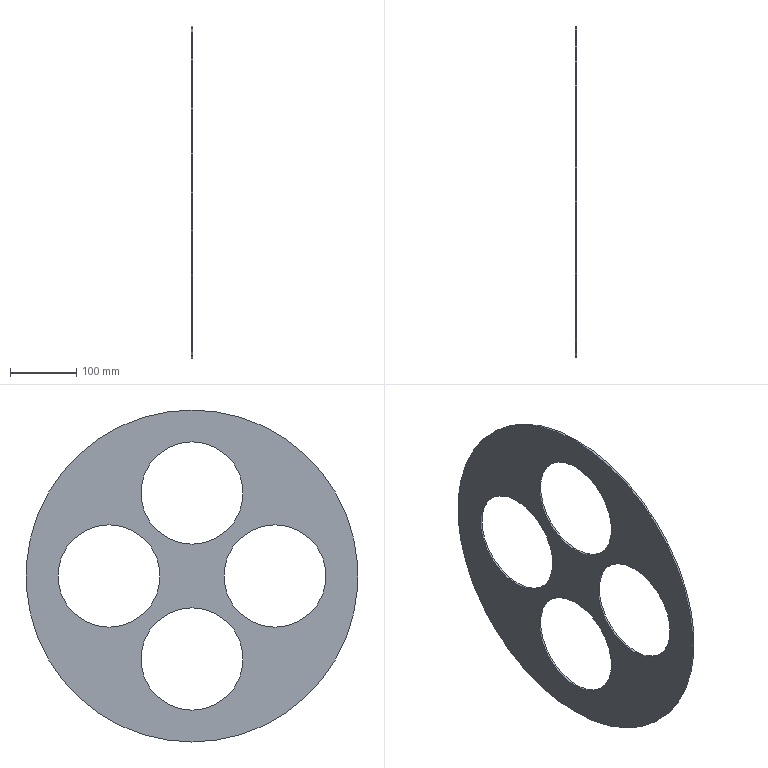Part | SolidWorks | features CirPattern 2, ICE 2, Extrusion 1 | 1 solid | 12 faces | box 3 x 500 x 500 mm | volume 365531 mm3 | cylinder 10 | plane 2 | commonest cylinder face diameters 154 x8 500 x2
STEP:
#1=CARTESIAN_POINT('',(0.,0.,-48.));
#2=VERTEX_POINT('',#1);
#3=CARTESIAN_POINT('',(0.,0.,-202.));
#4=VERTEX_POINT('',#3);
#5=CARTESIAN_POINT('',(0.,0.,-125.));
#6=DIRECTION('',(1.,0.,0.));
#7=DIRECTION('',(0.,0.,-1.));
#8=AXIS2_PLACEMENT_3D('',#5,#6,#7);
#9=CIRCLE('',#8,77.);
#10=EDGE_CURVE('',#2,#4,#9,.T.);
#11=ORIENTED_EDGE('',*,*,#10,.F.);
#12=CARTESIAN_POINT('',(3.,0.,-48.));
#13=VERTEX_POINT('',#12);
#14=CARTESIAN_POINT('',(-7.,0.,-48.));
#15=DIRECTION('',(1.,0.,0.));
#16=VECTOR('',#15,1000.);
#17=LINE('',#14,#16);
#18=EDGE_CURVE('',#2,#13,#17,.T.);
#19=ORIENTED_EDGE('',*,*,#18,.T.);
#20=CARTESIAN_POINT('',(3.,0.,-202.));
#21=VERTEX_POINT('',#20);
#22=CARTESIAN_POINT('',(3.,0.,-125.));
#23=DIRECTION('',(1.,0.,0.));
#24=DIRECTION('',(0.,-1.,0.));
#25=AXIS2_PLACEMENT_3D('',#22,#23,#24);
#26=CIRCLE('',#25,77.);
#27=EDGE_CURVE('',#13,#21,#26,.T.);
#28=ORIENTED_EDGE('',*,*,#27,.T.);
#29=CARTESIAN_POINT('',(-7.,0.,-202.));
#30=DIRECTION('',(1.,0.,0.));
#31=VECTOR('',#30,1000.);
#32=LINE('',#29,#31);
#33=EDGE_CURVE('',#4,#21,#32,.T.);
#34=ORIENTED_EDGE('',*,*,#33,.F.);
#35=EDGE_LOOP('',(#11,#19,#28,#34));
#36=FACE_OUTER_BOUND('',#35,.T.);
#37=CARTESIAN_POINT('',(-7.,0.,-125.));
#38=DIRECTION('',(1.,0.,0.));
#39=DIRECTION('',(0.,0.,-1.));
#40=AXIS2_PLACEMENT_3D('',#37,#38,#39);
#41=CYLINDRICAL_SURFACE('',#40,77.);
#42=ADVANCED_FACE('',(#36),#41,.F.);
#43=CARTESIAN_POINT('',(0.,-125.,77.));
#44=VERTEX_POINT('',#43);
#45=CARTESIAN_POINT('',(0.,-125.,-77.));
#46=VERTEX_POINT('',#45);
#47=CARTESIAN_POINT('',(0.,-125.,0.));
#48=DIRECTION('',(1.,0.,0.));
#49=DIRECTION('',(0.,0.,-1.));
#50=AXIS2_PLACEMENT_3D('',#47,#48,#49);
#51=CIRCLE('',#50,77.);
#52=EDGE_CURVE('',#44,#46,#51,.T.);
#53=ORIENTED_EDGE('',*,*,#52,.F.);
#54=CARTESIAN_POINT('',(3.,-125.,77.));
#55=VERTEX_POINT('',#54);
#56=CARTESIAN_POINT('',(-7.,-125.,77.));
#57=DIRECTION('',(1.,0.,0.));
#58=VECTOR('',#57,1000.);
#59=LINE('',#56,#58);
#60=EDGE_CURVE('',#44,#55,#59,.T.);
#61=ORIENTED_EDGE('',*,*,#60,.T.);
#62=CARTESIAN_POINT('',(3.,-125.,-77.));
#63=VERTEX_POINT('',#62);
#64=CARTESIAN_POINT('',(3.,-125.,0.));
#65=DIRECTION('',(1.,0.,0.));
#66=DIRECTION('',(0.,0.,1.));
#67=AXIS2_PLACEMENT_3D('',#64,#65,#66);
#68=CIRCLE('',#67,77.);
#69=EDGE_CURVE('',#55,#63,#68,.T.);
#70=ORIENTED_EDGE('',*,*,#69,.T.);
#71=CARTESIAN_POINT('',(-7.,-125.,-77.));
#72=DIRECTION('',(1.,0.,0.));
#73=VECTOR('',#72,1000.);
#74=LINE('',#71,#73);
#75=EDGE_CURVE('',#46,#63,#74,.T.);
#76=ORIENTED_EDGE('',*,*,#75,.F.);
#77=EDGE_LOOP('',(#53,#61,#70,#76));
#78=FACE_OUTER_BOUND('',#77,.T.);
#79=CARTESIAN_POINT('',(-7.,-125.,0.));
#80=DIRECTION('',(1.,0.,0.));
#81=DIRECTION('',(0.,0.,-1.));
#82=AXIS2_PLACEMENT_3D('',#79,#80,#81);
#83=CYLINDRICAL_SURFACE('',#82,77.);
#84=ADVANCED_FACE('',(#78),#83,.F.);
#85=CARTESIAN_POINT('',(0.,0.,202.));
#86=VERTEX_POINT('',#85);
#87=CARTESIAN_POINT('',(0.,0.,48.));
#88=VERTEX_POINT('',#87);
#89=CARTESIAN_POINT('',(0.,0.,125.));
#90=DIRECTION('',(1.,0.,0.));
#91=DIRECTION('',(0.,0.,-1.));
#92=AXIS2_PLACEMENT_3D('',#89,#90,#91);
#93=CIRCLE('',#92,77.);
#94=EDGE_CURVE('',#86,#88,#93,.T.);
#95=ORIENTED_EDGE('',*,*,#94,.F.);
#96=CARTESIAN_POINT('',(3.,0.,202.));
#97=VERTEX_POINT('',#96);
#98=CARTESIAN_POINT('',(-7.,0.,202.));
#99=DIRECTION('',(1.,0.,0.));
#100=VECTOR('',#99,1000.);
#101=LINE('',#98,#100);
#102=EDGE_CURVE('',#86,#97,#101,.T.);
#103=ORIENTED_EDGE('',*,*,#102,.T.);
#104=CARTESIAN_POINT('',(3.,0.,48.));
#105=VERTEX_POINT('',#104);
#106=CARTESIAN_POINT('',(3.,0.,125.));
#107=DIRECTION('',(1.,0.,0.));
#108=DIRECTION('',(0.,1.,0.));
#109=AXIS2_PLACEMENT_3D('',#106,#107,#108);
#110=CIRCLE('',#109,77.);
#111=EDGE_CURVE('',#97,#105,#110,.T.);
#112=ORIENTED_EDGE('',*,*,#111,.T.);
#113=CARTESIAN_POINT('',(-7.,0.,48.));
#114=DIRECTION('',(1.,0.,0.));
#115=VECTOR('',#114,1000.);
#116=LINE('',#113,#115);
#117=EDGE_CURVE('',#88,#105,#116,.T.);
#118=ORIENTED_EDGE('',*,*,#117,.F.);
#119=EDGE_LOOP('',(#95,#103,#112,#118));
#120=FACE_OUTER_BOUND('',#119,.T.);
#121=CARTESIAN_POINT('',(-7.,0.,125.));
#122=DIRECTION('',(1.,0.,0.));
#123=DIRECTION('',(0.,0.,-1.));
#124=AXIS2_PLACEMENT_3D('',#121,#122,#123);
#125=CYLINDRICAL_SURFACE('',#124,77.);
#126=ADVANCED_FACE('',(#120),#125,.F.);
#127=CARTESIAN_POINT('',(0.,125.,77.));
#128=VERTEX_POINT('',#127);
#129=CARTESIAN_POINT('',(0.,125.,-77.));
#130=VERTEX_POINT('',#129);
#131=CARTESIAN_POINT('',(0.,125.,0.));
#132=DIRECTION('',(1.,0.,0.));
#133=DIRECTION('',(0.,0.,-1.));
#134=AXIS2_PLACEMENT_3D('',#131,#132,#133);
#135=CIRCLE('',#134,77.);
#136=EDGE_CURVE('',#128,#130,#135,.T.);
#137=ORIENTED_EDGE('',*,*,#136,.F.);
#138=CARTESIAN_POINT('',(3.,125.,77.));
#139=VERTEX_POINT('',#138);
#140=CARTESIAN_POINT('',(-7.,125.,77.));
#141=DIRECTION('',(1.,0.,0.));
#142=VECTOR('',#141,1000.);
#143=LINE('',#140,#142);
#144=EDGE_CURVE('',#128,#139,#143,.T.);
#145=ORIENTED_EDGE('',*,*,#144,.T.);
#146=CARTESIAN_POINT('',(3.,125.,-77.));
#147=VERTEX_POINT('',#146);
#148=CARTESIAN_POINT('',(3.,125.,0.));
#149=DIRECTION('',(1.,0.,0.));
#150=DIRECTION('',(0.,0.,-1.));
#151=AXIS2_PLACEMENT_3D('',#148,#149,#150);
#152=CIRCLE('',#151,77.);
#153=EDGE_CURVE('',#139,#147,#152,.T.);
#154=ORIENTED_EDGE('',*,*,#153,.T.);
#155=CARTESIAN_POINT('',(-7.,125.,-77.));
#156=DIRECTION('',(1.,0.,0.));
#157=VECTOR('',#156,1000.);
#158=LINE('',#155,#157);
#159=EDGE_CURVE('',#130,#147,#158,.T.);
#160=ORIENTED_EDGE('',*,*,#159,.F.);
#161=EDGE_LOOP('',(#137,#145,#154,#160));
#162=FACE_OUTER_BOUND('',#161,.T.);
#163=CARTESIAN_POINT('',(-7.,125.,0.));
#164=DIRECTION('',(1.,0.,0.));
#165=DIRECTION('',(0.,0.,-1.));
#166=AXIS2_PLACEMENT_3D('',#163,#164,#165);
#167=CYLINDRICAL_SURFACE('',#166,77.);
#168=ADVANCED_FACE('',(#162),#167,.F.);
#169=CARTESIAN_POINT('',(3.,0.,-250.));
#170=VERTEX_POINT('',#169);
#171=CARTESIAN_POINT('',(3.,0.,250.));
#172=VERTEX_POINT('',#171);
#173=CARTESIAN_POINT('',(3.,0.,0.));
#174=DIRECTION('',(1.,0.,0.));
#175=DIRECTION('',(0.,0.,-1.));
#176=AXIS2_PLACEMENT_3D('',#173,#174,#175);
#177=CIRCLE('',#176,250.);
#178=EDGE_CURVE('',#170,#172,#177,.T.);
#179=ORIENTED_EDGE('',*,*,#178,.F.);
#180=CARTESIAN_POINT('',(0.,0.,-250.));
#181=VERTEX_POINT('',#180);
#182=CARTESIAN_POINT('',(3.,0.,-250.));
#183=DIRECTION('',(-1.,0.,0.));
#184=VECTOR('',#183,1000.);
#185=LINE('',#182,#184);
#186=EDGE_CURVE('',#170,#181,#185,.T.);
#187=ORIENTED_EDGE('',*,*,#186,.T.);
#188=CARTESIAN_POINT('',(0.,0.,250.));
#189=VERTEX_POINT('',#188);
#190=CARTESIAN_POINT('',(0.,0.,0.));
#191=DIRECTION('',(1.,0.,0.));
#192=DIRECTION('',(0.,0.,-1.));
#193=AXIS2_PLACEMENT_3D('',#190,#191,#192);
#194=CIRCLE('',#193,250.);
#195=EDGE_CURVE('',#181,#189,#194,.T.);
#196=ORIENTED_EDGE('',*,*,#195,.T.);
#197=CARTESIAN_POINT('',(3.,0.,250.));
#198=DIRECTION('',(-1.,0.,0.));
#199=VECTOR('',#198,1000.);
#200=LINE('',#197,#199);
#201=EDGE_CURVE('',#172,#189,#200,.T.);
#202=ORIENTED_EDGE('',*,*,#201,.F.);
#203=EDGE_LOOP('',(#179,#187,#196,#202));
#204=FACE_OUTER_BOUND('',#203,.T.);
#205=CARTESIAN_POINT('',(3.,0.,0.));
#206=DIRECTION('',(-1.,0.,0.));
#207=DIRECTION('',(0.,0.,1.));
#208=AXIS2_PLACEMENT_3D('',#205,#206,#207);
#209=CYLINDRICAL_SURFACE('',#208,250.);
#210=ADVANCED_FACE('',(#204),#209,.T.);
#211=ORIENTED_EDGE('',*,*,#186,.F.);
#212=CARTESIAN_POINT('',(3.,0.,0.));
#213=DIRECTION('',(1.,0.,0.));
#214=DIRECTION('',(0.,0.,-1.));
#215=AXIS2_PLACEMENT_3D('',#212,#213,#214);
#216=CIRCLE('',#215,250.);
#217=EDGE_CURVE('',#172,#170,#216,.T.);
#218=ORIENTED_EDGE('',*,*,#217,.F.);
#219=ORIENTED_EDGE('',*,*,#201,.T.);
#220=CARTESIAN_POINT('',(0.,0.,0.));
#221=DIRECTION('',(1.,0.,0.));
#222=DIRECTION('',(0.,0.,-1.));
#223=AXIS2_PLACEMENT_3D('',#220,#221,#222);
#224=CIRCLE('',#223,250.);
#225=EDGE_CURVE('',#189,#181,#224,.T.);
#226=ORIENTED_EDGE('',*,*,#225,.T.);
#227=EDGE_LOOP('',(#211,#218,#219,#226));
#228=FACE_OUTER_BOUND('',#227,.T.);
#229=CARTESIAN_POINT('',(3.,0.,0.));
#230=DIRECTION('',(-1.,0.,0.));
#231=DIRECTION('',(0.,0.,1.));
#232=AXIS2_PLACEMENT_3D('',#229,#230,#231);
#233=CYLINDRICAL_SURFACE('',#232,250.);
#234=ADVANCED_FACE('',(#228),#233,.T.);
#235=CARTESIAN_POINT('',(3.,0.,-125.));
#236=DIRECTION('',(1.,0.,0.));
#237=DIRECTION('',(0.,-1.,0.));
#238=AXIS2_PLACEMENT_3D('',#235,#236,#237);
#239=CIRCLE('',#238,77.);
#240=EDGE_CURVE('',#21,#13,#239,.T.);
#241=ORIENTED_EDGE('',*,*,#240,.F.);
#242=ORIENTED_EDGE('',*,*,#27,.F.);
#243=EDGE_LOOP('',(#241,#242));
#244=FACE_BOUND('',#243,.T.);
#245=CARTESIAN_POINT('',(3.,-125.,0.));
#246=DIRECTION('',(1.,0.,0.));
#247=DIRECTION('',(0.,0.,1.));
#248=AXIS2_PLACEMENT_3D('',#245,#246,#247);
#249=CIRCLE('',#248,77.);
#250=EDGE_CURVE('',#63,#55,#249,.T.);
#251=ORIENTED_EDGE('',*,*,#250,.F.);
#252=ORIENTED_EDGE('',*,*,#69,.F.);
#253=EDGE_LOOP('',(#251,#252));
#254=FACE_BOUND('',#253,.T.);
#255=CARTESIAN_POINT('',(3.,0.,125.));
#256=DIRECTION('',(1.,0.,0.));
#257=DIRECTION('',(0.,1.,0.));
#258=AXIS2_PLACEMENT_3D('',#255,#256,#257);
#259=CIRCLE('',#258,77.);
#260=EDGE_CURVE('',#105,#97,#259,.T.);
#261=ORIENTED_EDGE('',*,*,#260,.F.);
#262=ORIENTED_EDGE('',*,*,#111,.F.);
#263=EDGE_LOOP('',(#261,#262));
#264=FACE_BOUND('',#263,.T.);
#265=CARTESIAN_POINT('',(3.,125.,0.));
#266=DIRECTION('',(1.,0.,0.));
#267=DIRECTION('',(0.,0.,-1.));
#268=AXIS2_PLACEMENT_3D('',#265,#266,#267);
#269=CIRCLE('',#268,77.);
#270=EDGE_CURVE('',#147,#139,#269,.T.);
#271=ORIENTED_EDGE('',*,*,#270,.F.);
#272=ORIENTED_EDGE('',*,*,#153,.F.);
#273=EDGE_LOOP('',(#271,#272));
#274=FACE_BOUND('',#273,.T.);
#275=ORIENTED_EDGE('',*,*,#217,.T.);
#276=ORIENTED_EDGE('',*,*,#178,.T.);
#277=EDGE_LOOP('',(#275,#276));
#278=FACE_OUTER_BOUND('',#277,.T.);
#279=CARTESIAN_POINT('',(3.,0.,0.));
#280=DIRECTION('',(1.,0.,0.));
#281=DIRECTION('',(0.,0.,-1.));
#282=AXIS2_PLACEMENT_3D('',#279,#280,#281);
#283=PLANE('',#282);
#284=ADVANCED_FACE('',(#244,#254,#264,#274,#278),#283,.T.);
#285=CARTESIAN_POINT('',(0.,0.,-125.));
#286=DIRECTION('',(1.,0.,0.));
#287=DIRECTION('',(0.,0.,-1.));
#288=AXIS2_PLACEMENT_3D('',#285,#286,#287);
#289=CIRCLE('',#288,77.);
#290=EDGE_CURVE('',#4,#2,#289,.T.);
#291=ORIENTED_EDGE('',*,*,#290,.T.);
#292=ORIENTED_EDGE('',*,*,#10,.T.);
#293=EDGE_LOOP('',(#291,#292));
#294=FACE_BOUND('',#293,.T.);
#295=CARTESIAN_POINT('',(0.,-125.,0.));
#296=DIRECTION('',(1.,0.,0.));
#297=DIRECTION('',(0.,0.,-1.));
#298=AXIS2_PLACEMENT_3D('',#295,#296,#297);
#299=CIRCLE('',#298,77.);
#300=EDGE_CURVE('',#46,#44,#299,.T.);
#301=ORIENTED_EDGE('',*,*,#300,.T.);
#302=ORIENTED_EDGE('',*,*,#52,.T.);
#303=EDGE_LOOP('',(#301,#302));
#304=FACE_BOUND('',#303,.T.);
#305=CARTESIAN_POINT('',(0.,0.,125.));
#306=DIRECTION('',(1.,0.,0.));
#307=DIRECTION('',(0.,0.,-1.));
#308=AXIS2_PLACEMENT_3D('',#305,#306,#307);
#309=CIRCLE('',#308,77.);
#310=EDGE_CURVE('',#88,#86,#309,.T.);
#311=ORIENTED_EDGE('',*,*,#310,.T.);
#312=ORIENTED_EDGE('',*,*,#94,.T.);
#313=EDGE_LOOP('',(#311,#312));
#314=FACE_BOUND('',#313,.T.);
#315=CARTESIAN_POINT('',(0.,125.,0.));
#316=DIRECTION('',(1.,0.,0.));
#317=DIRECTION('',(0.,0.,-1.));
#318=AXIS2_PLACEMENT_3D('',#315,#316,#317);
#319=CIRCLE('',#318,77.);
#320=EDGE_CURVE('',#130,#128,#319,.T.);
#321=ORIENTED_EDGE('',*,*,#320,.T.);
#322=ORIENTED_EDGE('',*,*,#136,.T.);
#323=EDGE_LOOP('',(#321,#322));
#324=FACE_BOUND('',#323,.T.);
#325=ORIENTED_EDGE('',*,*,#225,.F.);
#326=ORIENTED_EDGE('',*,*,#195,.F.);
#327=EDGE_LOOP('',(#325,#326));
#328=FACE_OUTER_BOUND('',#327,.T.);
#329=CARTESIAN_POINT('',(0.,0.,0.));
#330=DIRECTION('',(1.,0.,0.));
#331=DIRECTION('',(0.,0.,-1.));
#332=AXIS2_PLACEMENT_3D('',#329,#330,#331);
#333=PLANE('',#332);
#334=ADVANCED_FACE('',(#294,#304,#314,#324,#328),#333,.F.);
#335=ORIENTED_EDGE('',*,*,#144,.F.);
#336=ORIENTED_EDGE('',*,*,#320,.F.);
#337=ORIENTED_EDGE('',*,*,#159,.T.);
#338=ORIENTED_EDGE('',*,*,#270,.T.);
#339=EDGE_LOOP('',(#335,#336,#337,#338));
#340=FACE_OUTER_BOUND('',#339,.T.);
#341=CARTESIAN_POINT('',(-7.,125.,0.));
#342=DIRECTION('',(1.,0.,0.));
#343=DIRECTION('',(0.,0.,-1.));
#344=AXIS2_PLACEMENT_3D('',#341,#342,#343);
#345=CYLINDRICAL_SURFACE('',#344,77.);
#346=ADVANCED_FACE('',(#340),#345,.F.);
#347=ORIENTED_EDGE('',*,*,#102,.F.);
#348=ORIENTED_EDGE('',*,*,#310,.F.);
#349=ORIENTED_EDGE('',*,*,#117,.T.);
#350=ORIENTED_EDGE('',*,*,#260,.T.);
#351=EDGE_LOOP('',(#347,#348,#349,#350));
#352=FACE_OUTER_BOUND('',#351,.T.);
#353=CARTESIAN_POINT('',(-7.,0.,125.));
#354=DIRECTION('',(1.,0.,0.));
#355=DIRECTION('',(0.,0.,-1.));
#356=AXIS2_PLACEMENT_3D('',#353,#354,#355);
#357=CYLINDRICAL_SURFACE('',#356,77.);
#358=ADVANCED_FACE('',(#352),#357,.F.);
#359=ORIENTED_EDGE('',*,*,#60,.F.);
#360=ORIENTED_EDGE('',*,*,#300,.F.);
#361=ORIENTED_EDGE('',*,*,#75,.T.);
#362=ORIENTED_EDGE('',*,*,#250,.T.);
#363=EDGE_LOOP('',(#359,#360,#361,#362));
#364=FACE_OUTER_BOUND('',#363,.T.);
#365=CARTESIAN_POINT('',(-7.,-125.,0.));
#366=DIRECTION('',(1.,0.,0.));
#367=DIRECTION('',(0.,0.,-1.));
#368=AXIS2_PLACEMENT_3D('',#365,#366,#367);
#369=CYLINDRICAL_SURFACE('',#368,77.);
#370=ADVANCED_FACE('',(#364),#369,.F.);
#371=ORIENTED_EDGE('',*,*,#18,.F.);
#372=ORIENTED_EDGE('',*,*,#290,.F.);
#373=ORIENTED_EDGE('',*,*,#33,.T.);
#374=ORIENTED_EDGE('',*,*,#240,.T.);
#375=EDGE_LOOP('',(#371,#372,#373,#374));
#376=FACE_OUTER_BOUND('',#375,.T.);
#377=CARTESIAN_POINT('',(-7.,0.,-125.));
#378=DIRECTION('',(1.,0.,0.));
#379=DIRECTION('',(0.,0.,-1.));
#380=AXIS2_PLACEMENT_3D('',#377,#378,#379);
#381=CYLINDRICAL_SURFACE('',#380,77.);
#382=ADVANCED_FACE('',(#376),#381,.F.);
#383=CLOSED_SHELL('',(#42,#84,#126,#168,#210,#234,#284,#334,#346,#358,#370,#382));
#384=MANIFOLD_SOLID_BREP('',#383);
#385=CARTESIAN_POINT('',(0.,0.,0.));
#386=DIRECTION('',(0.,0.,1.));
#387=DIRECTION('',(1.,0.,0.));
#388=AXIS2_PLACEMENT_3D('',#385,#386,#387);
#389=(LENGTH_UNIT()NAMED_UNIT(*)SI_UNIT(.MILLI.,.METRE.));
#390=UNCERTAINTY_MEASURE_WITH_UNIT(LENGTH_MEASURE(0.00001),#389,'','');
#391=(NAMED_UNIT(*)PLANE_ANGLE_UNIT()SI_UNIT($,.RADIAN.));
#392=(NAMED_UNIT(*)SI_UNIT($,.STERADIAN.)SOLID_ANGLE_UNIT());
#393=(GEOMETRIC_REPRESENTATION_CONTEXT(3)GLOBAL_UNCERTAINTY_ASSIGNED_CONTEXT((#390))GLOBAL_UNIT_ASSIGNED_CONTEXT((#389,#391,#392))REPRESENTATION_CONTEXT('',''));
#394=ADVANCED_BREP_SHAPE_REPRESENTATION('',(#384,#388),#393);